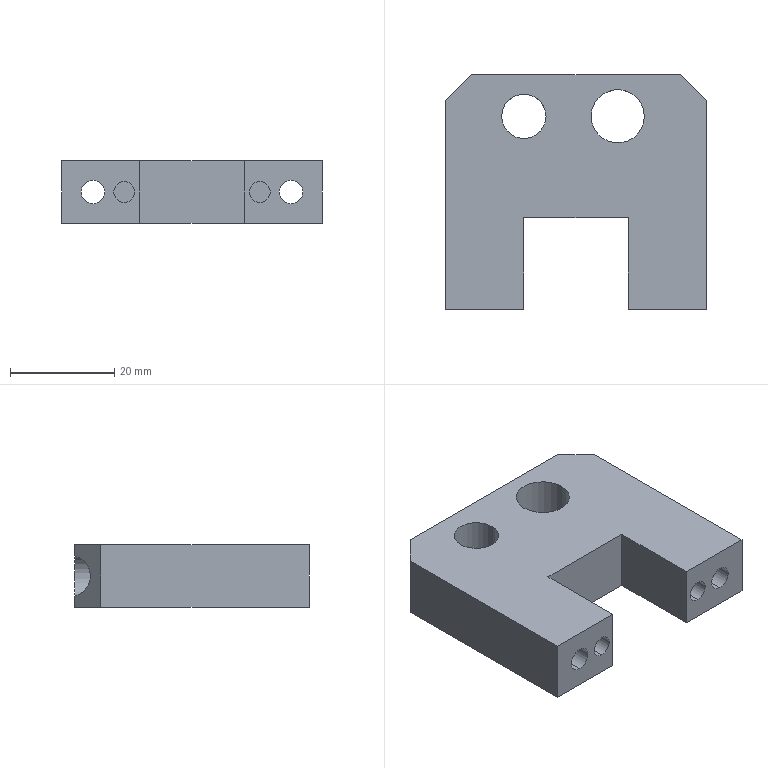Part | STEP file | PN_0010 | 1 solid | 32 faces | box 50 x 45 x 12 mm | volume 17113 mm3 | cylinder 16 | plane 16 | commonest cylinder face diameters 4 x4 4.5 x4 8 x4 8.5 x2 10.2 x2